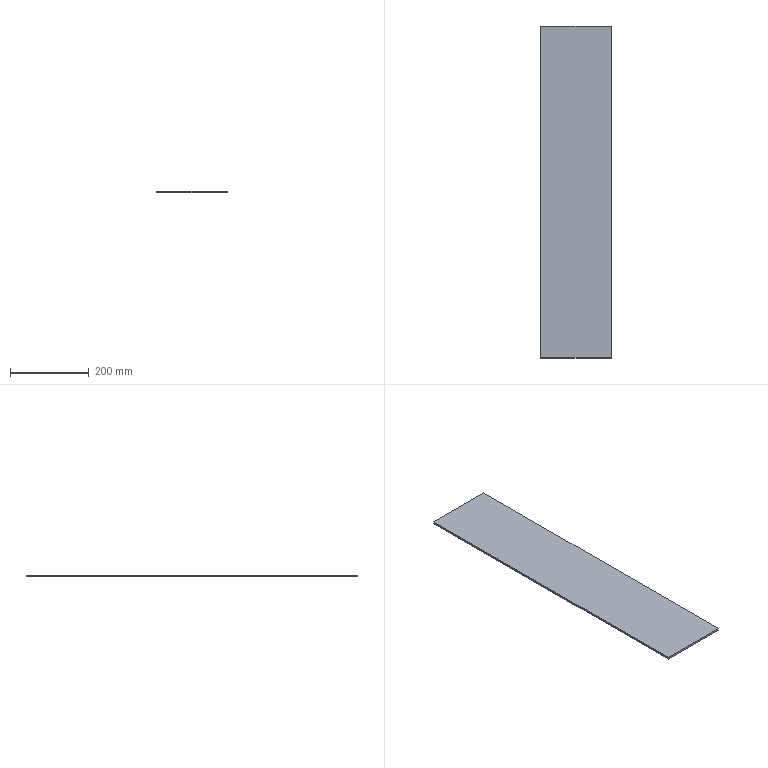Part | SolidWorks | features Extrusion 1, HoleWzd 1 | 1 solid | 6 faces | box 180 x 842 x 5 mm | volume 757800 mm3 | plane 6
STEP:
#1=CARTESIAN_POINT('',(90.,-421.,0.));
#2=VERTEX_POINT('',#1);
#3=CARTESIAN_POINT('',(90.,421.,0.));
#4=VERTEX_POINT('',#3);
#5=CARTESIAN_POINT('',(90.,421.,0.));
#6=DIRECTION('',(0.,1.,0.));
#7=VECTOR('',#6,1000.);
#8=LINE('',#5,#7);
#9=EDGE_CURVE('',#2,#4,#8,.T.);
#10=ORIENTED_EDGE('',*,*,#9,.T.);
#11=CARTESIAN_POINT('',(90.,421.,5.));
#12=VERTEX_POINT('',#11);
#13=CARTESIAN_POINT('',(90.,421.,5.));
#14=DIRECTION('',(0.,0.,-1.));
#15=VECTOR('',#14,1000.);
#16=LINE('',#13,#15);
#17=EDGE_CURVE('',#12,#4,#16,.T.);
#18=ORIENTED_EDGE('',*,*,#17,.F.);
#19=CARTESIAN_POINT('',(90.,-421.,5.));
#20=VERTEX_POINT('',#19);
#21=CARTESIAN_POINT('',(90.,421.,5.));
#22=DIRECTION('',(0.,1.,0.));
#23=VECTOR('',#22,1000.);
#24=LINE('',#21,#23);
#25=EDGE_CURVE('',#20,#12,#24,.T.);
#26=ORIENTED_EDGE('',*,*,#25,.F.);
#27=CARTESIAN_POINT('',(90.,-421.,5.));
#28=DIRECTION('',(0.,0.,-1.));
#29=VECTOR('',#28,1000.);
#30=LINE('',#27,#29);
#31=EDGE_CURVE('',#20,#2,#30,.T.);
#32=ORIENTED_EDGE('',*,*,#31,.T.);
#33=EDGE_LOOP('',(#10,#18,#26,#32));
#34=FACE_OUTER_BOUND('',#33,.T.);
#35=CARTESIAN_POINT('',(90.,421.,5.));
#36=DIRECTION('',(-1.,0.,0.));
#37=DIRECTION('',(0.,-1.,0.));
#38=AXIS2_PLACEMENT_3D('',#35,#36,#37);
#39=PLANE('',#38);
#40=ADVANCED_FACE('',(#34),#39,.F.);
#41=CARTESIAN_POINT('',(-90.,421.,0.));
#42=VERTEX_POINT('',#41);
#43=CARTESIAN_POINT('',(-90.,421.,0.));
#44=DIRECTION('',(-1.,0.,0.));
#45=VECTOR('',#44,1000.);
#46=LINE('',#43,#45);
#47=EDGE_CURVE('',#4,#42,#46,.T.);
#48=ORIENTED_EDGE('',*,*,#47,.T.);
#49=CARTESIAN_POINT('',(-90.,421.,5.));
#50=VERTEX_POINT('',#49);
#51=CARTESIAN_POINT('',(-90.,421.,5.));
#52=DIRECTION('',(0.,0.,-1.));
#53=VECTOR('',#52,1000.);
#54=LINE('',#51,#53);
#55=EDGE_CURVE('',#50,#42,#54,.T.);
#56=ORIENTED_EDGE('',*,*,#55,.F.);
#57=CARTESIAN_POINT('',(-90.,421.,5.));
#58=DIRECTION('',(-1.,0.,0.));
#59=VECTOR('',#58,1000.);
#60=LINE('',#57,#59);
#61=EDGE_CURVE('',#12,#50,#60,.T.);
#62=ORIENTED_EDGE('',*,*,#61,.F.);
#63=ORIENTED_EDGE('',*,*,#17,.T.);
#64=EDGE_LOOP('',(#48,#56,#62,#63));
#65=FACE_OUTER_BOUND('',#64,.T.);
#66=CARTESIAN_POINT('',(-90.,421.,5.));
#67=DIRECTION('',(0.,-1.,0.));
#68=DIRECTION('',(0.,0.,-1.));
#69=AXIS2_PLACEMENT_3D('',#66,#67,#68);
#70=PLANE('',#69);
#71=ADVANCED_FACE('',(#65),#70,.F.);
#72=CARTESIAN_POINT('',(-90.,-421.,0.));
#73=VERTEX_POINT('',#72);
#74=CARTESIAN_POINT('',(-90.,421.,0.));
#75=DIRECTION('',(0.,-1.,0.));
#76=VECTOR('',#75,1000.);
#77=LINE('',#74,#76);
#78=EDGE_CURVE('',#42,#73,#77,.T.);
#79=ORIENTED_EDGE('',*,*,#78,.T.);
#80=CARTESIAN_POINT('',(-90.,-421.,5.));
#81=VERTEX_POINT('',#80);
#82=CARTESIAN_POINT('',(-90.,-421.,5.));
#83=DIRECTION('',(0.,0.,-1.));
#84=VECTOR('',#83,1000.);
#85=LINE('',#82,#84);
#86=EDGE_CURVE('',#81,#73,#85,.T.);
#87=ORIENTED_EDGE('',*,*,#86,.F.);
#88=CARTESIAN_POINT('',(-90.,421.,5.));
#89=DIRECTION('',(0.,-1.,0.));
#90=VECTOR('',#89,1000.);
#91=LINE('',#88,#90);
#92=EDGE_CURVE('',#50,#81,#91,.T.);
#93=ORIENTED_EDGE('',*,*,#92,.F.);
#94=ORIENTED_EDGE('',*,*,#55,.T.);
#95=EDGE_LOOP('',(#79,#87,#93,#94));
#96=FACE_OUTER_BOUND('',#95,.T.);
#97=CARTESIAN_POINT('',(-90.,421.,5.));
#98=DIRECTION('',(1.,0.,0.));
#99=DIRECTION('',(0.,1.,0.));
#100=AXIS2_PLACEMENT_3D('',#97,#98,#99);
#101=PLANE('',#100);
#102=ADVANCED_FACE('',(#96),#101,.F.);
#103=CARTESIAN_POINT('',(-90.,-421.,0.));
#104=DIRECTION('',(1.,0.,0.));
#105=VECTOR('',#104,1000.);
#106=LINE('',#103,#105);
#107=EDGE_CURVE('',#73,#2,#106,.T.);
#108=ORIENTED_EDGE('',*,*,#107,.T.);
#109=ORIENTED_EDGE('',*,*,#31,.F.);
#110=CARTESIAN_POINT('',(-90.,-421.,5.));
#111=DIRECTION('',(1.,0.,0.));
#112=VECTOR('',#111,1000.);
#113=LINE('',#110,#112);
#114=EDGE_CURVE('',#81,#20,#113,.T.);
#115=ORIENTED_EDGE('',*,*,#114,.F.);
#116=ORIENTED_EDGE('',*,*,#86,.T.);
#117=EDGE_LOOP('',(#108,#109,#115,#116));
#118=FACE_OUTER_BOUND('',#117,.T.);
#119=CARTESIAN_POINT('',(-90.,-421.,5.));
#120=DIRECTION('',(0.,1.,0.));
#121=DIRECTION('',(0.,0.,1.));
#122=AXIS2_PLACEMENT_3D('',#119,#120,#121);
#123=PLANE('',#122);
#124=ADVANCED_FACE('',(#118),#123,.F.);
#125=ORIENTED_EDGE('',*,*,#25,.T.);
#126=ORIENTED_EDGE('',*,*,#61,.T.);
#127=ORIENTED_EDGE('',*,*,#92,.T.);
#128=ORIENTED_EDGE('',*,*,#114,.T.);
#129=EDGE_LOOP('',(#125,#126,#127,#128));
#130=FACE_OUTER_BOUND('',#129,.T.);
#131=CARTESIAN_POINT('',(0.,0.,5.));
#132=DIRECTION('',(0.,0.,1.));
#133=DIRECTION('',(1.,0.,0.));
#134=AXIS2_PLACEMENT_3D('',#131,#132,#133);
#135=PLANE('',#134);
#136=ADVANCED_FACE('',(#130),#135,.T.);
#137=ORIENTED_EDGE('',*,*,#9,.F.);
#138=ORIENTED_EDGE('',*,*,#107,.F.);
#139=ORIENTED_EDGE('',*,*,#78,.F.);
#140=ORIENTED_EDGE('',*,*,#47,.F.);
#141=EDGE_LOOP('',(#137,#138,#139,#140));
#142=FACE_OUTER_BOUND('',#141,.T.);
#143=CARTESIAN_POINT('',(0.,0.,0.));
#144=DIRECTION('',(0.,0.,1.));
#145=DIRECTION('',(1.,0.,0.));
#146=AXIS2_PLACEMENT_3D('',#143,#144,#145);
#147=PLANE('',#146);
#148=ADVANCED_FACE('',(#142),#147,.F.);
#149=CLOSED_SHELL('',(#40,#71,#102,#124,#136,#148));
#150=MANIFOLD_SOLID_BREP('',#149);
#151=CARTESIAN_POINT('',(0.,0.,0.));
#152=DIRECTION('',(0.,0.,1.));
#153=DIRECTION('',(1.,0.,0.));
#154=AXIS2_PLACEMENT_3D('',#151,#152,#153);
#155=(LENGTH_UNIT()NAMED_UNIT(*)SI_UNIT(.MILLI.,.METRE.));
#156=UNCERTAINTY_MEASURE_WITH_UNIT(LENGTH_MEASURE(0.00001),#155,'','');
#157=(NAMED_UNIT(*)PLANE_ANGLE_UNIT()SI_UNIT($,.RADIAN.));
#158=(NAMED_UNIT(*)SI_UNIT($,.STERADIAN.)SOLID_ANGLE_UNIT());
#159=(GEOMETRIC_REPRESENTATION_CONTEXT(3)GLOBAL_UNCERTAINTY_ASSIGNED_CONTEXT((#156))GLOBAL_UNIT_ASSIGNED_CONTEXT((#155,#157,#158))REPRESENTATION_CONTEXT('',''));
#160=ADVANCED_BREP_SHAPE_REPRESENTATION('',(#150,#154),#159);